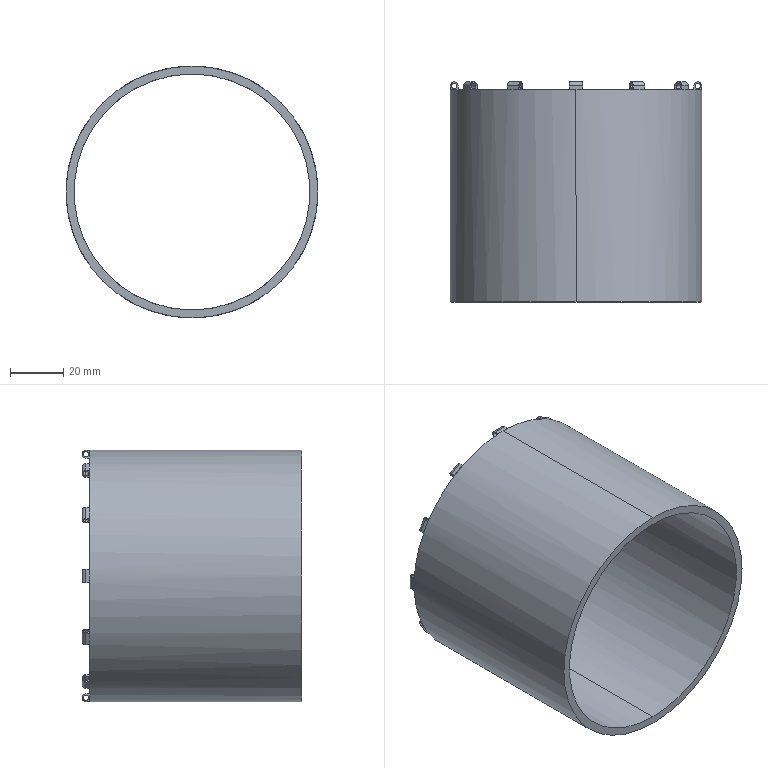Part | SolidWorks | features CirPattern 1, Extrusion 1, ICE 1 | 1 solid | 125 faces | box 95 x 83 x 95 mm | volume 69660 mm3 | plane 85 | cylinder 40 | commonest cylinder face diameters 2 x24 3 x12 89 x2 95 x2